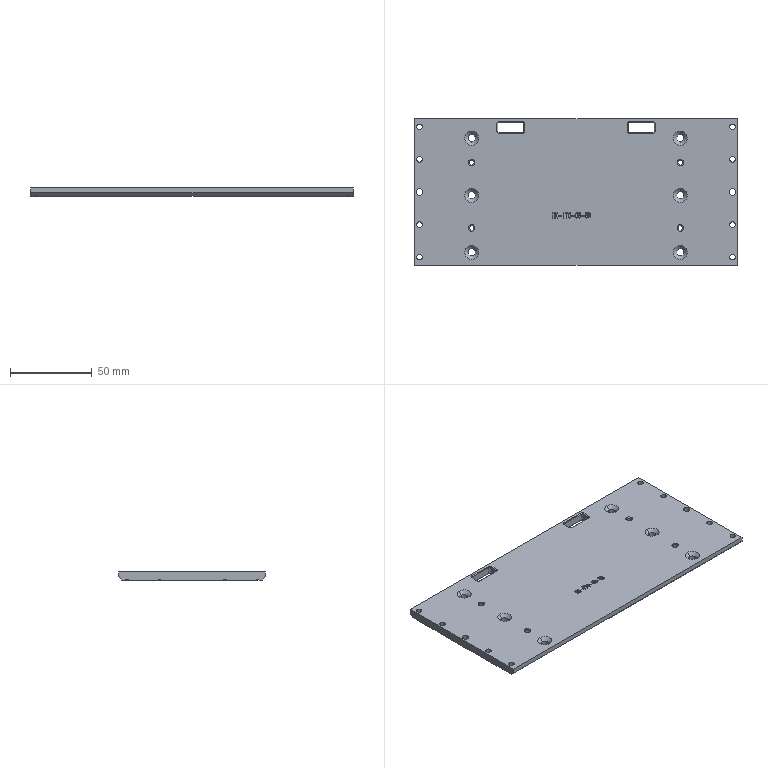NC program | NX | posted with a generic post | part box 198 x 90 x 5 mm
Lines 6815 to 7160 of 7160:
(刀补17 , TOOL : D2)
N13550 T17 M6
N13552 G54
N13554 G17 G0 G90 X-96. Y0. S9500 M3
N13556 G43 Z30. H17
N13558 Z0.5
N13560 G41 G94 G1 X-96.004 Y0.1 F1100. D17
N13562 G3 X-96.95 Y0. R0.478
N13564 X-96.95 Y0. Z-1.5 I0.95 J0.
N13566 X-96.95 Y0. Z-3.5 I0.95 J0.
N13568 X-96. Y0.95 Z-5. R-0.95
N13570 X-96.95 Y0. R0.95
N13572 X-96. Y0.95 R-0.95
N13574 X-96.1 Y0.004 R0.478
N13576 G40
N13578 G1 X-96. Y0.
N13580 G0 Z30.
N13582 X-64. Y18.
N13584 Z0.5
N13586 G41 G1 X-64.027 Y18.096
N13588 G3 X-64.45 Y18. R0.222
N13590 X-64.45 Y18. Z-1.5 I0.45 J0.
N13592 X-64.45 Y18. Z-3.5 I0.45 J0.
N13594 X-64. Y18.45 Z-5. R-0.45
N13596 X-64.45 Y18. R0.45
N13598 X-64. Y18.45 R-0.45
N13600 X-64.096 Y18.027 R0.222
N13602 G40
N13604 G1 X-64. Y18.
N13606 G0 Z30.
N13608 Y-22.
N13610 Z0.5
N13612 G41 G1 X-64.027 Y-21.904
N13614 G3 X-64.45 Y-22. R0.222
N13616 X-64.45 Y-22. Z-1.5 I0.45 J0.
N13618 X-64.45 Y-22. Z-3.5 I0.45 J0.
N13620 X-64. Y-21.55 Z-5. R-0.45
N13622 X-64.45 Y-22. R0.45
N13624 X-64. Y-21.55 R-0.45
N13626 X-64.096 Y-21.973 R0.222
N13628 G40
N13630 G1 X-64. Y-22.
N13632 G0 Z30.
N13634 X64.
N13636 Z0.5
N13638 G41 G1 X63.973 Y-21.904
N13640 G3 X63.55 Y-22. R0.222
N13642 X63.55 Y-22. Z-1.5 I0.45 J0.
N13644 X63.55 Y-22. Z-3.5 I0.45 J0.
N13646 X64. Y-21.55 Z-5. R-0.45
N13648 X63.55 Y-22. R0.45
N13650 X64. Y-21.55 R-0.45
N13652 X63.904 Y-21.973 R0.222
N13654 G40
N13656 G1 X64. Y-22.
N13658 G0 Z30.
N13660 X96. Y0.
N13662 Z0.5
N13664 G41 G1 X95.996 Y0.1
N13666 G3 X95.05 Y0. R0.478
N13668 X95.05 Y0. Z-1.5 I0.95 J0.
N13670 X95.05 Y0. Z-3.5 I0.95 J0.
N13672 X96. Y0.95 Z-5. R-0.95
N13674 X95.05 Y0. R0.95
N13676 X96. Y0.95 R-0.95
N13678 X95.9 Y0.004 R0.478
N13680 G40
N13682 G1 X96. Y0.
N13684 G0 Z30.
N13686 X64. Y18.
N13688 Z0.5
N13690 G41 G1 X63.973 Y18.096
N13692 G3 X63.55 Y18. R0.222
N13694 X63.55 Y18. Z-1.5 I0.45 J0.
N13696 X63.55 Y18. Z-3.5 I0.45 J0.
N13698 X64. Y18.45 Z-5. R-0.45
N13700 X63.55 Y18. R0.45
N13702 X64. Y18.45 R-0.45
N13704 X63.904 Y18.027 R0.222
N13706 G40
N13708 G1 X64. Y18.
N13710 G0 Z30.
N13712 M5
(ZLEVEL_PROFILE_COPY_1_COPY_COPY_1 , TOOL : D10JING)
N13714 T14 M6
N13716 G54
N13718 G17 G0 G90 X-100.622 Y51.809 S9500 M3
N13720 G43 Z30. H14
N13722 Z-3.525
N13724 G94 G1 Z-4.525 F1000.
N13726 X-99.866 Y50.5
N13728 G3 X-99. Y50. R1.
N13730 G1 X99. F1200.
N13732 G2 X104. Y45. R5.
N13734 G1 Y-45.
N13736 G2 X99. Y-50. R5.
N13738 G1 X-99.
N13740 G2 X-104. Y-45. R5.
N13742 G1 Y45.
N13744 G2 X-99. Y50. R5.
N13746 G1 X99. Z-4.566
N13748 X99.49 Y49.976
N13750 X99.975 Y49.904
N13752 X100.451 Y49.785
N13754 X100.913 Y49.619
N13756 X101.357 Y49.41
N13758 X101.778 Y49.157
N13760 X102.172 Y48.865
N13762 X102.536 Y48.536 Z-4.567
N13764 X102.865 Y48.172
N13766 X103.157 Y47.778
N13768 X103.41 Y47.357
N13770 X103.619 Y46.913
N13772 X103.785 Y46.451
N13774 X103.904 Y45.975
N13776 X103.976 Y45.49
N13778 X104. Y45.
N13780 X104.005 Y40.5 Z-4.568
N13782 X104. Y36. Z-4.569
N13784 Y-36. Z-4.584
N13786 X104.005 Y-40.5 Z-4.585
N13788 X104. Y-45. Z-4.586
N13790 X103.976 Y-45.49
N13792 X103.904 Y-45.975
N13794 X103.785 Y-46.451
N13796 X103.619 Y-46.913
N13798 X103.41 Y-47.357
N13800 X103.157 Y-47.778
N13802 X102.865 Y-48.172 Z-4.587
N13804 X102.536 Y-48.536
N13806 X102.172 Y-48.865
N13808 X101.778 Y-49.157
N13810 X101.357 Y-49.41
N13812 X100.913 Y-49.619
N13814 X100.451 Y-49.785
N13816 X99.975 Y-49.904
N13818 X99.49 Y-49.976
N13820 X99. Y-50. Z-4.588
N13822 X-99. Z-4.628
N13824 X-99.49 Y-49.976
N13826 X-99.975 Y-49.904
N13828 X-100.451 Y-49.785 Z-4.629
N13830 X-100.913 Y-49.619
N13832 X-101.357 Y-49.41
N13834 X-101.778 Y-49.157
N13836 X-102.172 Y-48.865
N13838 X-102.536 Y-48.536
N13840 X-102.865 Y-48.172
N13842 X-103.157 Y-47.778
N13844 X-103.41 Y-47.357
N13846 X-103.619 Y-46.913
N13848 X-103.785 Y-46.451 Z-4.63
N13850 X-103.904 Y-45.975
N13852 X-103.976 Y-45.49
N13854 X-104. Y-45.
N13856 X-104.003 Y-40. Z-4.631
N13858 X-104. Y-35. Z-4.632
N13860 Y35. Z-4.646
N13862 X-104.003 Y40. Z-4.647
N13864 X-104. Y45. Z-4.648
N13866 X-103.976 Y45.49
N13868 X-103.904 Y45.975 Z-4.649
N13870 X-103.785 Y46.451
N13872 X-103.619 Y46.913
N13874 X-103.41 Y47.357
N13876 X-103.157 Y47.778
N13878 X-102.865 Y48.172
N13880 X-102.536 Y48.536
N13882 X-102.172 Y48.865
N13884 X-101.778 Y49.157
N13886 X-101.357 Y49.41
N13888 X-100.913 Y49.619 Z-4.65
N13890 X-100.451 Y49.785
N13892 X-99.975 Y49.904
N13894 X-99.49 Y49.976
N13896 X-99. Y50.
N13898 X99. Z-4.691
N13900 X99.49 Y49.976
N13902 X99.975 Y49.904
N13904 X100.451 Y49.785
N13906 X100.913 Y49.619
N13908 X101.357 Y49.41
N13910 X101.778 Y49.157
N13912 X102.172 Y48.865
N13914 X102.536 Y48.536 Z-4.692
N13916 X102.865 Y48.172
N13918 X103.157 Y47.778
N13920 X103.41 Y47.357
N13922 X103.619 Y46.913
N13924 X103.785 Y46.451
N13926 X103.904 Y45.975
N13928 X103.976 Y45.49
N13930 X104. Y45.
N13932 X104.005 Y40.5 Z-4.693
N13934 X104. Y36. Z-4.694
N13936 Y-36. Z-4.709
N13938 X104.005 Y-40.5 Z-4.71
N13940 X104. Y-45. Z-4.711
N13942 X103.976 Y-45.49
N13944 X103.904 Y-45.975
N13946 X103.785 Y-46.451
N13948 X103.619 Y-46.913
N13950 X103.41 Y-47.357
N13952 X103.157 Y-47.778
N13954 X102.865 Y-48.172 Z-4.712
N13956 X102.536 Y-48.536
N13958 X102.172 Y-48.865
N13960 X101.778 Y-49.157
N13962 X101.357 Y-49.41
N13964 X100.913 Y-49.619
N13966 X100.451 Y-49.785
N13968 X99.975 Y-49.904
N13970 X99.49 Y-49.976
N13972 X99. Y-50. Z-4.713
N13974 X-99. Z-4.753
N13976 X-99.49 Y-49.976
N13978 X-99.975 Y-49.904
N13980 X-100.451 Y-49.785 Z-4.754
N13982 X-100.913 Y-49.619
N13984 X-101.357 Y-49.41
N13986 X-101.778 Y-49.157
N13988 X-102.172 Y-48.865
N13990 X-102.536 Y-48.536
N13992 X-102.865 Y-48.172
N13994 X-103.157 Y-47.778
N13996 X-103.41 Y-47.357
N13998 X-103.619 Y-46.913
N14000 X-103.785 Y-46.451 Z-4.755
N14002 X-103.904 Y-45.975
N14004 X-103.976 Y-45.49
N14006 X-104. Y-45.
N14008 X-104.003 Y-40. Z-4.756
N14010 X-104. Y-35. Z-4.757
N14012 Y35. Z-4.771
N14014 X-104.003 Y40. Z-4.772
N14016 X-104. Y45. Z-4.773
N14018 X-103.976 Y45.49
N14020 X-103.904 Y45.975 Z-4.774
N14022 X-103.785 Y46.451
N14024 X-103.619 Y46.913
N14026 X-103.41 Y47.357
N14028 X-103.157 Y47.778
N14030 X-102.865 Y48.172
N14032 X-102.536 Y48.536
N14034 X-102.172 Y48.865
N14036 X-101.778 Y49.157
N14038 X-101.357 Y49.41
N14040 X-100.913 Y49.619 Z-4.775
N14042 X-100.451 Y49.785
N14044 X-99.975 Y49.904
N14046 X-99.49 Y49.976
N14048 X-99. Y50.
N14050 X99. Z-4.816
N14052 X99.49 Y49.976
N14054 X99.975 Y49.904
N14056 X100.451 Y49.785
N14058 X100.913 Y49.619
N14060 X101.357 Y49.41
N14062 X101.778 Y49.157
N14064 X102.172 Y48.865
N14066 X102.536 Y48.536 Z-4.817
N14068 X102.865 Y48.172
N14070 X103.157 Y47.778
N14072 X103.41 Y47.357
N14074 X103.619 Y46.913
N14076 X103.785 Y46.451
N14078 X103.904 Y45.975
N14080 X103.976 Y45.49
N14082 X104. Y45.
N14084 X104.005 Y40.5 Z-4.818
N14086 X104. Y36. Z-4.819
N14088 Y-36. Z-4.834
N14090 X104.005 Y-40.5 Z-4.835
N14092 X104. Y-45. Z-4.836
N14094 X103.976 Y-45.49
N14096 X103.904 Y-45.975
N14098 X103.785 Y-46.451
N14100 X103.619 Y-46.913
N14102 X103.41 Y-47.357
N14104 X103.157 Y-47.778
N14106 X102.865 Y-48.172 Z-4.837
N14108 X102.536 Y-48.536
N14110 X102.172 Y-48.865
N14112 X101.778 Y-49.157
N14114 X101.357 Y-49.41
N14116 X100.913 Y-49.619
N14118 X100.451 Y-49.785
N14120 X99.975 Y-49.904
N14122 X99.49 Y-49.976
N14124 X99. Y-50. Z-4.838
N14126 X-99. Z-4.878
N14128 X-99.49 Y-49.976
N14130 X-99.975 Y-49.904
N14132 X-100.451 Y-49.785 Z-4.879
N14134 X-100.913 Y-49.619
N14136 X-101.357 Y-49.41
N14138 X-101.778 Y-49.157
N14140 X-102.172 Y-48.865
N14142 X-102.536 Y-48.536
N14144 X-102.865 Y-48.172
N14146 X-103.157 Y-47.778
N14148 X-103.41 Y-47.357
N14150 X-103.619 Y-46.913
N14152 X-103.785 Y-46.451 Z-4.88
N14154 X-103.904 Y-45.975
N14156 X-103.976 Y-45.49
N14158 X-104. Y-45.
N14160 X-104.003 Y-40. Z-4.881
N14162 X-104. Y-35. Z-4.882
N14164 Y35. Z-4.896
N14166 X-104.003 Y40. Z-4.897
N14168 X-104. Y45. Z-4.898
N14170 X-103.976 Y45.49
N14172 X-103.904 Y45.975 Z-4.899
N14174 X-103.785 Y46.451
N14176 X-103.619 Y46.913
N14178 X-103.41 Y47.357
N14180 X-103.157 Y47.778
N14182 X-102.865 Y48.172
N14184 X-102.536 Y48.536
N14186 X-102.172 Y48.865
N14188 X-101.778 Y49.157
N14190 X-101.357 Y49.41
N14192 X-100.913 Y49.619 Z-4.9
N14194 X-100.451 Y49.785
N14196 X-99.975 Y49.904
N14198 X-99.49 Y49.976
N14200 X-99. Y50.
N14202 X99.
N14204 G2 X104. Y45. R5.
N14206 G1 Y-45.
N14208 G2 X99. Y-50. R5.
N14210 G1 X-99.
N14212 G2 X-104. Y-45. R5.
N14214 G1 Y45.
N14216 G2 X-99. Y50. R5.
N14218 G3 X-98.134 Y50.5 R1.
N14220 G1 X-97.268 Y52.
N14222 Z-3.9
N14224 G0 Z30.
N14226 M5
N14228 M2